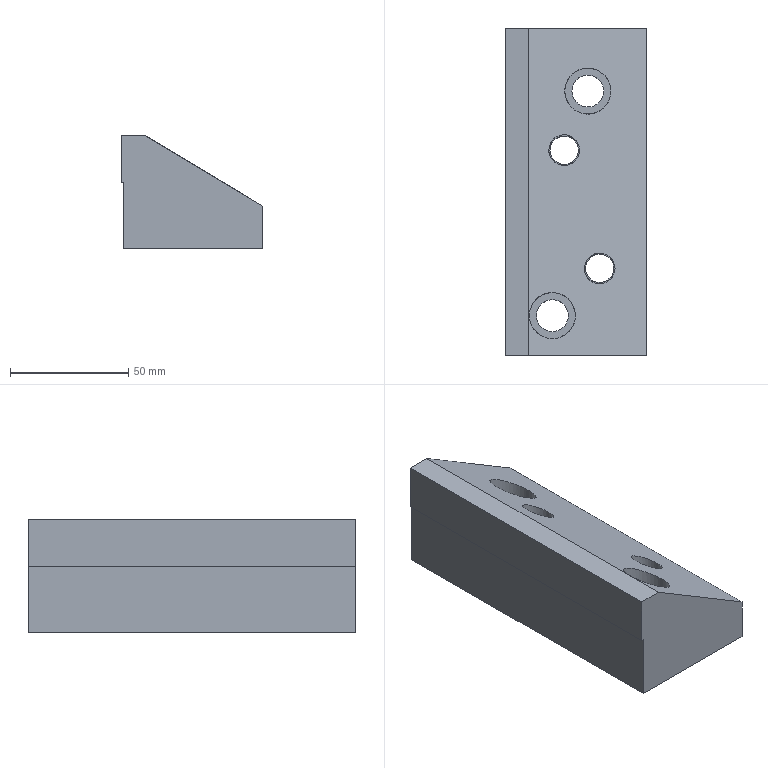Part | NX | features solid 2 | 1 solid | 21 faces | box 60 x 138.619 x 48 mm | volume 266827 mm3 | plane 13 | cylinder 8 | commonest cylinder face diameters 12 x2 13 x2 13.5 x2 19.5 x2
STEP:
#1=CARTESIAN_POINT('',(-70.,-232.,-27.));
#2=VERTEX_POINT('',#1);
#3=CARTESIAN_POINT('',(-69.,-232.,-27.));
#4=VERTEX_POINT('',#3);
#5=CARTESIAN_POINT('',(-70.,-232.,-27.));
#6=DIRECTION('',(-1.,0.,0.));
#7=VECTOR('',#6,1000.);
#8=LINE('',#5,#7);
#9=EDGE_CURVE('',#2,#4,#8,.F.);
#10=ORIENTED_EDGE('',*,*,#9,.T.);
#11=CARTESIAN_POINT('',(-69.,-232.,-55.));
#12=VERTEX_POINT('',#11);
#13=CARTESIAN_POINT('',(-69.,-232.,-27.));
#14=DIRECTION('',(0.,0.,-1.));
#15=VECTOR('',#14,1000.);
#16=LINE('',#13,#15);
#17=EDGE_CURVE('',#4,#12,#16,.T.);
#18=ORIENTED_EDGE('',*,*,#17,.T.);
#19=CARTESIAN_POINT('',(-10.,-232.,-55.));
#20=VERTEX_POINT('',#19);
#21=CARTESIAN_POINT('',(-70.,-232.,-55.));
#22=DIRECTION('',(-1.,0.,0.));
#23=VECTOR('',#22,1000.);
#24=LINE('',#21,#23);
#25=EDGE_CURVE('',#12,#20,#24,.F.);
#26=ORIENTED_EDGE('',*,*,#25,.T.);
#27=CARTESIAN_POINT('',(-10.,-232.,-37.));
#28=VERTEX_POINT('',#27);
#29=CARTESIAN_POINT('',(-10.,-232.,-67.));
#30=DIRECTION('',(0.,0.,1.));
#31=VECTOR('',#30,1000.);
#32=LINE('',#29,#31);
#33=EDGE_CURVE('',#20,#28,#32,.T.);
#34=ORIENTED_EDGE('',*,*,#33,.T.);
#35=CARTESIAN_POINT('',(-60.,-232.,-7.));
#36=VERTEX_POINT('',#35);
#37=CARTESIAN_POINT('',(-40.882,-232.,-18.471));
#38=DIRECTION('',(0.8575,0.,-0.5145));
#39=VECTOR('',#38,1000.);
#40=LINE('',#37,#39);
#41=EDGE_CURVE('',#28,#36,#40,.F.);
#42=ORIENTED_EDGE('',*,*,#41,.T.);
#43=CARTESIAN_POINT('',(-70.,-232.,-7.));
#44=VERTEX_POINT('',#43);
#45=CARTESIAN_POINT('',(-70.,-232.,-7.));
#46=DIRECTION('',(-1.,0.,0.));
#47=VECTOR('',#46,1000.);
#48=LINE('',#45,#47);
#49=EDGE_CURVE('',#44,#36,#48,.F.);
#50=ORIENTED_EDGE('',*,*,#49,.F.);
#51=CARTESIAN_POINT('',(-70.,-232.,-67.));
#52=DIRECTION('',(0.,0.,1.));
#53=VECTOR('',#52,1000.);
#54=LINE('',#51,#53);
#55=EDGE_CURVE('',#2,#44,#54,.T.);
#56=ORIENTED_EDGE('',*,*,#55,.F.);
#57=EDGE_LOOP('',(#10,#18,#26,#34,#42,#50,#56));
#58=FACE_BOUND('',#57,.T.);
#59=CARTESIAN_POINT('',(-70.,-232.,-67.));
#60=DIRECTION('',(0.,-1.,0.));
#61=DIRECTION('',(0.,0.,1.));
#62=AXIS2_PLACEMENT_3D('',#59,#60,#61);
#63=PLANE('',#62);
#64=ADVANCED_FACE('',(#58),#63,.T.);
#65=CARTESIAN_POINT('',(-70.,-93.381,-27.));
#66=VERTEX_POINT('',#65);
#67=CARTESIAN_POINT('',(-69.,-93.381,-27.));
#68=VERTEX_POINT('',#67);
#69=CARTESIAN_POINT('',(-70.,-93.381,-27.));
#70=DIRECTION('',(-1.,0.,0.));
#71=VECTOR('',#70,1000.);
#72=LINE('',#69,#71);
#73=EDGE_CURVE('',#66,#68,#72,.F.);
#74=ORIENTED_EDGE('',*,*,#73,.F.);
#75=CARTESIAN_POINT('',(-70.,-93.381,-7.));
#76=VERTEX_POINT('',#75);
#77=CARTESIAN_POINT('',(-70.,-93.381,-67.));
#78=DIRECTION('',(0.,0.,1.));
#79=VECTOR('',#78,1000.);
#80=LINE('',#77,#79);
#81=EDGE_CURVE('',#66,#76,#80,.T.);
#82=ORIENTED_EDGE('',*,*,#81,.T.);
#83=CARTESIAN_POINT('',(-60.,-93.381,-7.));
#84=VERTEX_POINT('',#83);
#85=CARTESIAN_POINT('',(-70.,-93.381,-7.));
#86=DIRECTION('',(1.,0.,0.));
#87=VECTOR('',#86,1000.);
#88=LINE('',#85,#87);
#89=EDGE_CURVE('',#76,#84,#88,.T.);
#90=ORIENTED_EDGE('',*,*,#89,.T.);
#91=CARTESIAN_POINT('',(-10.,-93.381,-37.));
#92=VERTEX_POINT('',#91);
#93=CARTESIAN_POINT('',(-40.882,-93.381,-18.471));
#94=DIRECTION('',(0.8575,0.,-0.5145));
#95=VECTOR('',#94,1000.);
#96=LINE('',#93,#95);
#97=EDGE_CURVE('',#84,#92,#96,.T.);
#98=ORIENTED_EDGE('',*,*,#97,.T.);
#99=CARTESIAN_POINT('',(-10.,-93.381,-55.));
#100=VERTEX_POINT('',#99);
#101=CARTESIAN_POINT('',(-10.,-93.381,-67.));
#102=DIRECTION('',(0.,0.,1.));
#103=VECTOR('',#102,1000.);
#104=LINE('',#101,#103);
#105=EDGE_CURVE('',#100,#92,#104,.T.);
#106=ORIENTED_EDGE('',*,*,#105,.F.);
#107=CARTESIAN_POINT('',(-69.,-93.381,-55.));
#108=VERTEX_POINT('',#107);
#109=CARTESIAN_POINT('',(-415.478,-93.381,-55.));
#110=DIRECTION('',(1.,0.,0.));
#111=VECTOR('',#110,1000.);
#112=LINE('',#109,#111);
#113=EDGE_CURVE('',#108,#100,#112,.T.);
#114=ORIENTED_EDGE('',*,*,#113,.F.);
#115=CARTESIAN_POINT('',(-69.,-93.381,-27.));
#116=DIRECTION('',(0.,0.,-1.));
#117=VECTOR('',#116,1000.);
#118=LINE('',#115,#117);
#119=EDGE_CURVE('',#68,#108,#118,.T.);
#120=ORIENTED_EDGE('',*,*,#119,.F.);
#121=EDGE_LOOP('',(#74,#82,#90,#98,#106,#114,#120));
#122=FACE_BOUND('',#121,.T.);
#123=CARTESIAN_POINT('',(-70.,-93.381,-67.));
#124=DIRECTION('',(0.,-1.,0.));
#125=DIRECTION('',(0.,0.,1.));
#126=AXIS2_PLACEMENT_3D('',#123,#124,#125);
#127=PLANE('',#126);
#128=ADVANCED_FACE('',(#122),#127,.F.);
#129=ORIENTED_EDGE('',*,*,#81,.F.);
#130=CARTESIAN_POINT('',(-70.,-99.381,-27.));
#131=DIRECTION('',(0.,1.,0.));
#132=VECTOR('',#131,1000.);
#133=LINE('',#130,#132);
#134=EDGE_CURVE('',#66,#2,#133,.F.);
#135=ORIENTED_EDGE('',*,*,#134,.T.);
#136=ORIENTED_EDGE('',*,*,#55,.T.);
#137=CARTESIAN_POINT('',(-70.,-99.381,-7.));
#138=DIRECTION('',(0.,-1.,0.));
#139=VECTOR('',#138,1000.);
#140=LINE('',#137,#139);
#141=EDGE_CURVE('',#76,#44,#140,.T.);
#142=ORIENTED_EDGE('',*,*,#141,.F.);
#143=EDGE_LOOP('',(#129,#135,#136,#142));
#144=FACE_BOUND('',#143,.T.);
#145=CARTESIAN_POINT('',(-70.,-99.381,-67.));
#146=DIRECTION('',(-1.,0.,0.));
#147=DIRECTION('',(0.,0.,1.));
#148=AXIS2_PLACEMENT_3D('',#145,#146,#147);
#149=PLANE('',#148);
#150=ADVANCED_FACE('',(#144),#149,.T.);
#151=CARTESIAN_POINT('',(-24.,-195.,-55.));
#152=VERTEX_POINT('',#151);
#153=CARTESIAN_POINT('',(-30.,-195.,-55.));
#154=DIRECTION('',(0.,0.,1.));
#155=DIRECTION('',(1.,0.,0.));
#156=AXIS2_PLACEMENT_3D('',#153,#154,#155);
#157=CIRCLE('',#156,6.);
#158=EDGE_CURVE('',#152,#152,#157,.T.);
#159=ORIENTED_EDGE('',*,*,#158,.T.);
#160=EDGE_LOOP('',(#159));
#161=FACE_BOUND('',#160,.T.);
#162=CARTESIAN_POINT('',(-39.,-145.,-55.));
#163=VERTEX_POINT('',#162);
#164=CARTESIAN_POINT('',(-45.,-145.,-55.));
#165=DIRECTION('',(0.,0.,1.));
#166=DIRECTION('',(1.,0.,0.));
#167=AXIS2_PLACEMENT_3D('',#164,#165,#166);
#168=CIRCLE('',#167,6.);
#169=EDGE_CURVE('',#163,#163,#168,.T.);
#170=ORIENTED_EDGE('',*,*,#169,.T.);
#171=EDGE_LOOP('',(#170));
#172=FACE_BOUND('',#171,.T.);
#173=CARTESIAN_POINT('',(-43.25,-215.,-55.));
#174=VERTEX_POINT('',#173);
#175=CARTESIAN_POINT('',(-50.,-215.,-55.));
#176=DIRECTION('',(0.,0.,1.));
#177=DIRECTION('',(1.,0.,0.));
#178=AXIS2_PLACEMENT_3D('',#175,#176,#177);
#179=CIRCLE('',#178,6.75);
#180=EDGE_CURVE('',#174,#174,#179,.T.);
#181=ORIENTED_EDGE('',*,*,#180,.T.);
#182=EDGE_LOOP('',(#181));
#183=FACE_BOUND('',#182,.T.);
#184=CARTESIAN_POINT('',(-28.25,-120.,-55.));
#185=VERTEX_POINT('',#184);
#186=CARTESIAN_POINT('',(-35.,-120.,-55.));
#187=DIRECTION('',(0.,0.,1.));
#188=DIRECTION('',(1.,0.,0.));
#189=AXIS2_PLACEMENT_3D('',#186,#187,#188);
#190=CIRCLE('',#189,6.75);
#191=EDGE_CURVE('',#185,#185,#190,.T.);
#192=ORIENTED_EDGE('',*,*,#191,.T.);
#193=EDGE_LOOP('',(#192));
#194=FACE_BOUND('',#193,.T.);
#195=ORIENTED_EDGE('',*,*,#25,.F.);
#196=CARTESIAN_POINT('',(-69.,35.09,-55.));
#197=DIRECTION('',(0.,1.,0.));
#198=VECTOR('',#197,1000.);
#199=LINE('',#196,#198);
#200=EDGE_CURVE('',#12,#108,#199,.T.);
#201=ORIENTED_EDGE('',*,*,#200,.T.);
#202=ORIENTED_EDGE('',*,*,#113,.T.);
#203=CARTESIAN_POINT('',(-10.,35.09,-55.));
#204=DIRECTION('',(0.,-1.,0.));
#205=VECTOR('',#204,1000.);
#206=LINE('',#203,#205);
#207=EDGE_CURVE('',#100,#20,#206,.T.);
#208=ORIENTED_EDGE('',*,*,#207,.T.);
#209=EDGE_LOOP('',(#195,#201,#202,#208));
#210=FACE_BOUND('',#209,.T.);
#211=CARTESIAN_POINT('',(-415.478,35.09,-55.));
#212=DIRECTION('',(0.,0.,1.));
#213=DIRECTION('',(1.,0.,0.));
#214=AXIS2_PLACEMENT_3D('',#211,#212,#213);
#215=PLANE('',#214);
#216=ADVANCED_FACE('',(#161,#172,#183,#194,#210),#215,.F.);
#217=ORIENTED_EDGE('',*,*,#49,.T.);
#218=CARTESIAN_POINT('',(-60.,-99.381,-7.));
#219=DIRECTION('',(0.,1.,0.));
#220=VECTOR('',#219,1000.);
#221=LINE('',#218,#220);
#222=EDGE_CURVE('',#36,#84,#221,.T.);
#223=ORIENTED_EDGE('',*,*,#222,.T.);
#224=ORIENTED_EDGE('',*,*,#89,.F.);
#225=ORIENTED_EDGE('',*,*,#141,.T.);
#226=EDGE_LOOP('',(#217,#223,#224,#225));
#227=FACE_BOUND('',#226,.T.);
#228=CARTESIAN_POINT('',(-70.,-99.381,-7.));
#229=DIRECTION('',(0.,0.,-1.));
#230=DIRECTION('',(0.,-1.,0.));
#231=AXIS2_PLACEMENT_3D('',#228,#229,#230);
#232=PLANE('',#231);
#233=ADVANCED_FACE('',(#227),#232,.F.);
#234=ORIENTED_EDGE('',*,*,#105,.T.);
#235=CARTESIAN_POINT('',(-10.,-99.381,-37.));
#236=DIRECTION('',(0.,-1.,0.));
#237=VECTOR('',#236,1000.);
#238=LINE('',#235,#237);
#239=EDGE_CURVE('',#92,#28,#238,.T.);
#240=ORIENTED_EDGE('',*,*,#239,.T.);
#241=ORIENTED_EDGE('',*,*,#33,.F.);
#242=ORIENTED_EDGE('',*,*,#207,.F.);
#243=EDGE_LOOP('',(#234,#240,#241,#242));
#244=FACE_BOUND('',#243,.T.);
#245=CARTESIAN_POINT('',(-10.,-99.381,-67.));
#246=DIRECTION('',(-1.,0.,0.));
#247=DIRECTION('',(0.,0.,1.));
#248=AXIS2_PLACEMENT_3D('',#245,#246,#247);
#249=PLANE('',#248);
#250=ADVANCED_FACE('',(#244),#249,.F.);
#251=CARTESIAN_POINT('',(-36.5,-195.,-21.1));
#252=VERTEX_POINT('',#251);
#253=CARTESIAN_POINT('',(-30.,-195.,-25.));
#254=DIRECTION('',(-0.5145,0.,-0.8575));
#255=DIRECTION('',(-0.8575,0.,0.5145));
#256=AXIS2_PLACEMENT_3D('',#253,#254,#255);
#257=ELLIPSE('',#256,7.58,6.5);
#258=EDGE_CURVE('',#252,#252,#257,.T.);
#259=ORIENTED_EDGE('',*,*,#258,.T.);
#260=EDGE_LOOP('',(#259));
#261=FACE_BOUND('',#260,.T.);
#262=CARTESIAN_POINT('',(-51.5,-145.,-12.1));
#263=VERTEX_POINT('',#262);
#264=CARTESIAN_POINT('',(-45.,-145.,-16.));
#265=DIRECTION('',(-0.5145,0.,-0.8575));
#266=DIRECTION('',(-0.8575,0.,0.5145));
#267=AXIS2_PLACEMENT_3D('',#264,#265,#266);
#268=ELLIPSE('',#267,7.58,6.5);
#269=EDGE_CURVE('',#263,#263,#268,.T.);
#270=ORIENTED_EDGE('',*,*,#269,.T.);
#271=EDGE_LOOP('',(#270));
#272=FACE_BOUND('',#271,.T.);
#273=CARTESIAN_POINT('',(-59.75,-215.,-7.15));
#274=VERTEX_POINT('',#273);
#275=CARTESIAN_POINT('',(-50.,-215.,-13.));
#276=DIRECTION('',(-0.5145,0.,-0.8575));
#277=DIRECTION('',(-0.8575,0.,0.5145));
#278=AXIS2_PLACEMENT_3D('',#275,#276,#277);
#279=ELLIPSE('',#278,11.37,9.75);
#280=EDGE_CURVE('',#274,#274,#279,.T.);
#281=ORIENTED_EDGE('',*,*,#280,.T.);
#282=EDGE_LOOP('',(#281));
#283=FACE_BOUND('',#282,.T.);
#284=CARTESIAN_POINT('',(-44.75,-120.,-16.15));
#285=VERTEX_POINT('',#284);
#286=CARTESIAN_POINT('',(-35.,-120.,-22.));
#287=DIRECTION('',(-0.5145,0.,-0.8575));
#288=DIRECTION('',(-0.8575,0.,0.5145));
#289=AXIS2_PLACEMENT_3D('',#286,#287,#288);
#290=ELLIPSE('',#289,11.37,9.75);
#291=EDGE_CURVE('',#285,#285,#290,.T.);
#292=ORIENTED_EDGE('',*,*,#291,.T.);
#293=EDGE_LOOP('',(#292));
#294=FACE_BOUND('',#293,.T.);
#295=ORIENTED_EDGE('',*,*,#41,.F.);
#296=ORIENTED_EDGE('',*,*,#239,.F.);
#297=ORIENTED_EDGE('',*,*,#97,.F.);
#298=ORIENTED_EDGE('',*,*,#222,.F.);
#299=EDGE_LOOP('',(#295,#296,#297,#298));
#300=FACE_BOUND('',#299,.T.);
#301=CARTESIAN_POINT('',(-60.,-232.,-7.));
#302=DIRECTION('',(-0.5145,0.,-0.8575));
#303=DIRECTION('',(-0.8575,0.,0.5145));
#304=AXIS2_PLACEMENT_3D('',#301,#302,#303);
#305=PLANE('',#304);
#306=ADVANCED_FACE('',(#261,#272,#283,#294,#300),#305,.F.);
#307=ORIENTED_EDGE('',*,*,#17,.F.);
#308=CARTESIAN_POINT('',(-69.,-99.381,-27.));
#309=DIRECTION('',(0.,1.,0.));
#310=VECTOR('',#309,1000.);
#311=LINE('',#308,#310);
#312=EDGE_CURVE('',#68,#4,#311,.F.);
#313=ORIENTED_EDGE('',*,*,#312,.F.);
#314=ORIENTED_EDGE('',*,*,#119,.T.);
#315=ORIENTED_EDGE('',*,*,#200,.F.);
#316=EDGE_LOOP('',(#307,#313,#314,#315));
#317=FACE_BOUND('',#316,.T.);
#318=CARTESIAN_POINT('',(-69.,-99.381,-27.));
#319=DIRECTION('',(1.,0.,0.));
#320=DIRECTION('',(0.,0.,-1.));
#321=AXIS2_PLACEMENT_3D('',#318,#319,#320);
#322=PLANE('',#321);
#323=ADVANCED_FACE('',(#317),#322,.F.);
#324=ORIENTED_EDGE('',*,*,#73,.T.);
#325=ORIENTED_EDGE('',*,*,#312,.T.);
#326=ORIENTED_EDGE('',*,*,#9,.F.);
#327=ORIENTED_EDGE('',*,*,#134,.F.);
#328=EDGE_LOOP('',(#324,#325,#326,#327));
#329=FACE_BOUND('',#328,.T.);
#330=CARTESIAN_POINT('',(-70.,-99.381,-27.));
#331=DIRECTION('',(0.,0.,1.));
#332=DIRECTION('',(0.,-1.,0.));
#333=AXIS2_PLACEMENT_3D('',#330,#331,#332);
#334=PLANE('',#333);
#335=ADVANCED_FACE('',(#329),#334,.F.);
#336=CARTESIAN_POINT('',(-41.75,-120.,-35.));
#337=VERTEX_POINT('',#336);
#338=CARTESIAN_POINT('',(-35.,-120.,-35.));
#339=DIRECTION('',(0.,0.,-1.));
#340=DIRECTION('',(-1.,0.,0.));
#341=AXIS2_PLACEMENT_3D('',#338,#339,#340);
#342=CIRCLE('',#341,6.75);
#343=EDGE_CURVE('',#337,#337,#342,.F.);
#344=ORIENTED_EDGE('',*,*,#343,.T.);
#345=EDGE_LOOP('',(#344));
#346=FACE_BOUND('',#345,.T.);
#347=ORIENTED_EDGE('',*,*,#191,.F.);
#348=EDGE_LOOP('',(#347));
#349=FACE_BOUND('',#348,.T.);
#350=CARTESIAN_POINT('',(-35.,-120.,-75.));
#351=DIRECTION('',(0.,0.,1.));
#352=DIRECTION('',(1.,0.,0.));
#353=AXIS2_PLACEMENT_3D('',#350,#351,#352);
#354=CYLINDRICAL_SURFACE('',#353,6.75);
#355=ADVANCED_FACE('',(#346,#349),#354,.F.);
#356=CARTESIAN_POINT('',(-25.25,-120.,-35.));
#357=VERTEX_POINT('',#356);
#358=CARTESIAN_POINT('',(-35.,-120.,-35.));
#359=DIRECTION('',(0.,0.,1.));
#360=DIRECTION('',(1.,0.,0.));
#361=AXIS2_PLACEMENT_3D('',#358,#359,#360);
#362=CIRCLE('',#361,9.75);
#363=EDGE_CURVE('',#357,#357,#362,.T.);
#364=ORIENTED_EDGE('',*,*,#363,.F.);
#365=EDGE_LOOP('',(#364));
#366=FACE_BOUND('',#365,.T.);
#367=ORIENTED_EDGE('',*,*,#291,.F.);
#368=EDGE_LOOP('',(#367));
#369=FACE_BOUND('',#368,.T.);
#370=CARTESIAN_POINT('',(-35.,-120.,-35.));
#371=DIRECTION('',(0.,0.,1.));
#372=DIRECTION('',(1.,0.,0.));
#373=AXIS2_PLACEMENT_3D('',#370,#371,#372);
#374=CYLINDRICAL_SURFACE('',#373,9.75);
#375=ADVANCED_FACE('',(#366,#369),#374,.F.);
#376=ORIENTED_EDGE('',*,*,#343,.F.);
#377=EDGE_LOOP('',(#376));
#378=FACE_BOUND('',#377,.T.);
#379=ORIENTED_EDGE('',*,*,#363,.T.);
#380=EDGE_LOOP('',(#379));
#381=FACE_BOUND('',#380,.T.);
#382=CARTESIAN_POINT('',(-35.,-125.,-35.));
#383=DIRECTION('',(0.,0.,-1.));
#384=DIRECTION('',(-1.,0.,0.));
#385=AXIS2_PLACEMENT_3D('',#382,#383,#384);
#386=PLANE('',#385);
#387=ADVANCED_FACE('',(#378,#381),#386,.F.);
#388=CARTESIAN_POINT('',(-56.75,-215.,-35.));
#389=VERTEX_POINT('',#388);
#390=CARTESIAN_POINT('',(-50.,-215.,-35.));
#391=DIRECTION('',(0.,0.,-1.));
#392=DIRECTION('',(-1.,0.,0.));
#393=AXIS2_PLACEMENT_3D('',#390,#391,#392);
#394=CIRCLE('',#393,6.75);
#395=EDGE_CURVE('',#389,#389,#394,.F.);
#396=ORIENTED_EDGE('',*,*,#395,.T.);
#397=EDGE_LOOP('',(#396));
#398=FACE_BOUND('',#397,.T.);
#399=ORIENTED_EDGE('',*,*,#180,.F.);
#400=EDGE_LOOP('',(#399));
#401=FACE_BOUND('',#400,.T.);
#402=CARTESIAN_POINT('',(-50.,-215.,-75.));
#403=DIRECTION('',(0.,0.,1.));
#404=DIRECTION('',(1.,0.,0.));
#405=AXIS2_PLACEMENT_3D('',#402,#403,#404);
#406=CYLINDRICAL_SURFACE('',#405,6.75);
#407=ADVANCED_FACE('',(#398,#401),#406,.F.);
#408=CARTESIAN_POINT('',(-40.25,-215.,-35.));
#409=VERTEX_POINT('',#408);
#410=CARTESIAN_POINT('',(-50.,-215.,-35.));
#411=DIRECTION('',(0.,0.,1.));
#412=DIRECTION('',(1.,0.,0.));
#413=AXIS2_PLACEMENT_3D('',#410,#411,#412);
#414=CIRCLE('',#413,9.75);
#415=EDGE_CURVE('',#409,#409,#414,.T.);
#416=ORIENTED_EDGE('',*,*,#415,.F.);
#417=EDGE_LOOP('',(#416));
#418=FACE_BOUND('',#417,.T.);
#419=ORIENTED_EDGE('',*,*,#280,.F.);
#420=EDGE_LOOP('',(#419));
#421=FACE_BOUND('',#420,.T.);
#422=CARTESIAN_POINT('',(-50.,-215.,-35.));
#423=DIRECTION('',(0.,0.,1.));
#424=DIRECTION('',(1.,0.,0.));
#425=AXIS2_PLACEMENT_3D('',#422,#423,#424);
#426=CYLINDRICAL_SURFACE('',#425,9.75);
#427=ADVANCED_FACE('',(#418,#421),#426,.F.);
#428=ORIENTED_EDGE('',*,*,#395,.F.);
#429=EDGE_LOOP('',(#428));
#430=FACE_BOUND('',#429,.T.);
#431=ORIENTED_EDGE('',*,*,#415,.T.);
#432=EDGE_LOOP('',(#431));
#433=FACE_BOUND('',#432,.T.);
#434=CARTESIAN_POINT('',(-50.,-215.,-35.));
#435=DIRECTION('',(0.,0.,-1.));
#436=DIRECTION('',(-1.,0.,0.));
#437=AXIS2_PLACEMENT_3D('',#434,#435,#436);
#438=PLANE('',#437);
#439=ADVANCED_FACE('',(#430,#433),#438,.F.);
#440=CARTESIAN_POINT('',(-51.,-145.,-35.));
#441=VERTEX_POINT('',#440);
#442=CARTESIAN_POINT('',(-45.,-145.,-35.));
#443=DIRECTION('',(0.,0.,-1.));
#444=DIRECTION('',(-1.,0.,0.));
#445=AXIS2_PLACEMENT_3D('',#442,#443,#444);
#446=CIRCLE('',#445,6.);
#447=EDGE_CURVE('',#441,#441,#446,.F.);
#448=ORIENTED_EDGE('',*,*,#447,.T.);
#449=EDGE_LOOP('',(#448));
#450=FACE_BOUND('',#449,.T.);
#451=ORIENTED_EDGE('',*,*,#169,.F.);
#452=EDGE_LOOP('',(#451));
#453=FACE_BOUND('',#452,.T.);
#454=CARTESIAN_POINT('',(-45.,-145.,-75.));
#455=DIRECTION('',(0.,0.,1.));
#456=DIRECTION('',(1.,0.,0.));
#457=AXIS2_PLACEMENT_3D('',#454,#455,#456);
#458=CYLINDRICAL_SURFACE('',#457,6.);
#459=ADVANCED_FACE('',(#450,#453),#458,.F.);
#460=CARTESIAN_POINT('',(-38.5,-145.,-35.));
#461=VERTEX_POINT('',#460);
#462=CARTESIAN_POINT('',(-45.,-145.,-35.));
#463=DIRECTION('',(0.,0.,1.));
#464=DIRECTION('',(1.,0.,0.));
#465=AXIS2_PLACEMENT_3D('',#462,#463,#464);
#466=CIRCLE('',#465,6.5);
#467=EDGE_CURVE('',#461,#461,#466,.T.);
#468=ORIENTED_EDGE('',*,*,#467,.F.);
#469=EDGE_LOOP('',(#468));
#470=FACE_BOUND('',#469,.T.);
#471=ORIENTED_EDGE('',*,*,#269,.F.);
#472=EDGE_LOOP('',(#471));
#473=FACE_BOUND('',#472,.T.);
#474=CARTESIAN_POINT('',(-45.,-145.,-35.));
#475=DIRECTION('',(0.,0.,1.));
#476=DIRECTION('',(1.,0.,0.));
#477=AXIS2_PLACEMENT_3D('',#474,#475,#476);
#478=CYLINDRICAL_SURFACE('',#477,6.5);
#479=ADVANCED_FACE('',(#470,#473),#478,.F.);
#480=ORIENTED_EDGE('',*,*,#447,.F.);
#481=EDGE_LOOP('',(#480));
#482=FACE_BOUND('',#481,.T.);
#483=ORIENTED_EDGE('',*,*,#467,.T.);
#484=EDGE_LOOP('',(#483));
#485=FACE_BOUND('',#484,.T.);
#486=CARTESIAN_POINT('',(-50.,-145.,-35.));
#487=DIRECTION('',(0.,0.,-1.));
#488=DIRECTION('',(-1.,0.,0.));
#489=AXIS2_PLACEMENT_3D('',#486,#487,#488);
#490=PLANE('',#489);
#491=ADVANCED_FACE('',(#482,#485),#490,.F.);
#492=CARTESIAN_POINT('',(-36.,-195.,-35.));
#493=VERTEX_POINT('',#492);
#494=CARTESIAN_POINT('',(-30.,-195.,-35.));
#495=DIRECTION('',(0.,0.,-1.));
#496=DIRECTION('',(-1.,0.,0.));
#497=AXIS2_PLACEMENT_3D('',#494,#495,#496);
#498=CIRCLE('',#497,6.);
#499=EDGE_CURVE('',#493,#493,#498,.F.);
#500=ORIENTED_EDGE('',*,*,#499,.T.);
#501=EDGE_LOOP('',(#500));
#502=FACE_BOUND('',#501,.T.);
#503=ORIENTED_EDGE('',*,*,#158,.F.);
#504=EDGE_LOOP('',(#503));
#505=FACE_BOUND('',#504,.T.);
#506=CARTESIAN_POINT('',(-30.,-195.,-75.));
#507=DIRECTION('',(0.,0.,1.));
#508=DIRECTION('',(1.,0.,0.));
#509=AXIS2_PLACEMENT_3D('',#506,#507,#508);
#510=CYLINDRICAL_SURFACE('',#509,6.);
#511=ADVANCED_FACE('',(#502,#505),#510,.F.);
#512=CARTESIAN_POINT('',(-23.5,-195.,-35.));
#513=VERTEX_POINT('',#512);
#514=CARTESIAN_POINT('',(-30.,-195.,-35.));
#515=DIRECTION('',(0.,0.,1.));
#516=DIRECTION('',(1.,0.,0.));
#517=AXIS2_PLACEMENT_3D('',#514,#515,#516);
#518=CIRCLE('',#517,6.5);
#519=EDGE_CURVE('',#513,#513,#518,.T.);
#520=ORIENTED_EDGE('',*,*,#519,.F.);
#521=EDGE_LOOP('',(#520));
#522=FACE_BOUND('',#521,.T.);
#523=ORIENTED_EDGE('',*,*,#258,.F.);
#524=EDGE_LOOP('',(#523));
#525=FACE_BOUND('',#524,.T.);
#526=CARTESIAN_POINT('',(-30.,-195.,-35.));
#527=DIRECTION('',(0.,0.,1.));
#528=DIRECTION('',(1.,0.,0.));
#529=AXIS2_PLACEMENT_3D('',#526,#527,#528);
#530=CYLINDRICAL_SURFACE('',#529,6.5);
#531=ADVANCED_FACE('',(#522,#525),#530,.F.);
#532=ORIENTED_EDGE('',*,*,#499,.F.);
#533=EDGE_LOOP('',(#532));
#534=FACE_BOUND('',#533,.T.);
#535=ORIENTED_EDGE('',*,*,#519,.T.);
#536=EDGE_LOOP('',(#535));
#537=FACE_BOUND('',#536,.T.);
#538=CARTESIAN_POINT('',(-35.,-195.,-35.));
#539=DIRECTION('',(0.,0.,-1.));
#540=DIRECTION('',(-1.,0.,0.));
#541=AXIS2_PLACEMENT_3D('',#538,#539,#540);
#542=PLANE('',#541);
#543=ADVANCED_FACE('',(#534,#537),#542,.F.);
#544=CLOSED_SHELL('',(#64,#128,#150,#216,#233,#250,#306,#323,#335,#355,#375,#387,#407,#427,#439,#459,#479,#491,#511,#531,#543));
#545=MANIFOLD_SOLID_BREP('',#544);
#546=(LENGTH_UNIT()NAMED_UNIT(*)SI_UNIT(.MILLI.,.METRE.));
#547=UNCERTAINTY_MEASURE_WITH_UNIT(LENGTH_MEASURE(0.00001),#546,'','');
#548=(NAMED_UNIT(*)PLANE_ANGLE_UNIT()SI_UNIT($,.RADIAN.));
#549=(NAMED_UNIT(*)SI_UNIT($,.STERADIAN.)SOLID_ANGLE_UNIT());
#550=(GEOMETRIC_REPRESENTATION_CONTEXT(3)GLOBAL_UNCERTAINTY_ASSIGNED_CONTEXT((#547))GLOBAL_UNIT_ASSIGNED_CONTEXT((#546,#548,#549))REPRESENTATION_CONTEXT('',''));
#551=ADVANCED_BREP_SHAPE_REPRESENTATION('',(#545),#550);